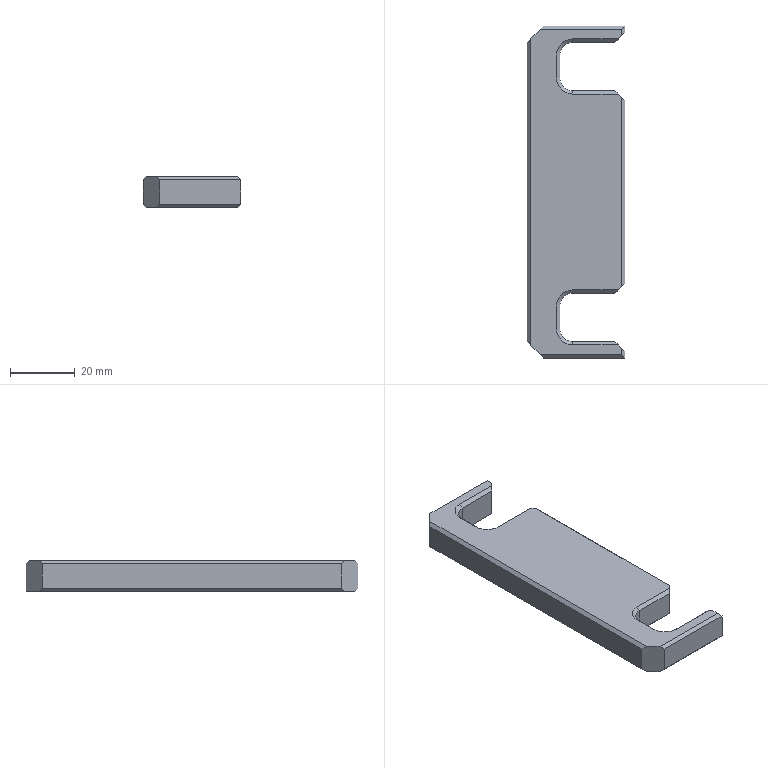Part | NX | features CHAMFER 3, DATUM_CSYS 3, EXTRUDE 3, BLEND 2, EXTRACT_STRING 2, SKETCH 2, Instance Feature 1, Pattern Feature 1 | 1 solid | 50 faces | box 30 x 102.4 x 9.5 mm | volume 22943 mm3 | plane 40 | cone 6 | cylinder 4 | commonest cylinder face diameters 8 x4
STEP:
#1=CARTESIAN_POINT('',(30.,23.,1.));
#2=VERTEX_POINT('',#1);
#3=CARTESIAN_POINT('',(30.,79.4,1.));
#4=VERTEX_POINT('',#3);
#5=CARTESIAN_POINT('',(30.,0.,1.));
#6=DIRECTION('',(0.,1.,0.));
#7=VECTOR('',#6,1000.);
#8=LINE('',#5,#7);
#9=EDGE_CURVE('',#2,#4,#8,.T.);
#10=ORIENTED_EDGE('',*,*,#9,.T.);
#11=CARTESIAN_POINT('',(30.,79.4,8.5));
#12=VERTEX_POINT('',#11);
#13=CARTESIAN_POINT('',(30.,79.4,8.5));
#14=DIRECTION('',(0.,0.,1.));
#15=VECTOR('',#14,1000.);
#16=LINE('',#13,#15);
#17=EDGE_CURVE('',#4,#12,#16,.T.);
#18=ORIENTED_EDGE('',*,*,#17,.T.);
#19=CARTESIAN_POINT('',(30.,23.,8.5));
#20=VERTEX_POINT('',#19);
#21=CARTESIAN_POINT('',(30.,0.,8.5));
#22=DIRECTION('',(0.,-1.,0.));
#23=VECTOR('',#22,1000.);
#24=LINE('',#21,#23);
#25=EDGE_CURVE('',#12,#20,#24,.T.);
#26=ORIENTED_EDGE('',*,*,#25,.T.);
#27=CARTESIAN_POINT('',(30.,23.,1.));
#28=DIRECTION('',(0.,0.,-1.));
#29=VECTOR('',#28,1000.);
#30=LINE('',#27,#29);
#31=EDGE_CURVE('',#20,#2,#30,.T.);
#32=ORIENTED_EDGE('',*,*,#31,.T.);
#33=EDGE_LOOP('',(#10,#18,#26,#32));
#34=FACE_BOUND('',#33,.T.);
#35=CARTESIAN_POINT('',(30.,0.,0.));
#36=DIRECTION('',(1.,0.,0.));
#37=DIRECTION('',(0.,0.,-1.));
#38=AXIS2_PLACEMENT_3D('',#35,#36,#37);
#39=PLANE('',#38);
#40=ADVANCED_FACE('',(#34),#39,.T.);
#41=CARTESIAN_POINT('',(30.,0.,1.));
#42=VERTEX_POINT('',#41);
#43=CARTESIAN_POINT('',(30.,2.,1.));
#44=VERTEX_POINT('',#43);
#45=CARTESIAN_POINT('',(30.,0.,1.));
#46=DIRECTION('',(0.,1.,0.));
#47=VECTOR('',#46,1000.);
#48=LINE('',#45,#47);
#49=EDGE_CURVE('',#42,#44,#48,.T.);
#50=ORIENTED_EDGE('',*,*,#49,.T.);
#51=CARTESIAN_POINT('',(30.,2.,8.5));
#52=VERTEX_POINT('',#51);
#53=CARTESIAN_POINT('',(30.,2.,8.5));
#54=DIRECTION('',(0.,0.,1.));
#55=VECTOR('',#54,1000.);
#56=LINE('',#53,#55);
#57=EDGE_CURVE('',#44,#52,#56,.T.);
#58=ORIENTED_EDGE('',*,*,#57,.T.);
#59=CARTESIAN_POINT('',(30.,0.,8.5));
#60=VERTEX_POINT('',#59);
#61=CARTESIAN_POINT('',(30.,0.,8.5));
#62=DIRECTION('',(0.,-1.,0.));
#63=VECTOR('',#62,1000.);
#64=LINE('',#61,#63);
#65=EDGE_CURVE('',#52,#60,#64,.T.);
#66=ORIENTED_EDGE('',*,*,#65,.T.);
#67=CARTESIAN_POINT('',(30.,0.,9.5));
#68=DIRECTION('',(0.,0.,-1.));
#69=VECTOR('',#68,1000.);
#70=LINE('',#67,#69);
#71=EDGE_CURVE('',#60,#42,#70,.T.);
#72=ORIENTED_EDGE('',*,*,#71,.T.);
#73=EDGE_LOOP('',(#50,#58,#66,#72));
#74=FACE_BOUND('',#73,.T.);
#75=CARTESIAN_POINT('',(30.,0.,0.));
#76=DIRECTION('',(1.,0.,0.));
#77=DIRECTION('',(0.,0.,-1.));
#78=AXIS2_PLACEMENT_3D('',#75,#76,#77);
#79=PLANE('',#78);
#80=ADVANCED_FACE('',(#74),#79,.T.);
#81=CARTESIAN_POINT('',(5.,0.,8.5));
#82=VERTEX_POINT('',#81);
#83=CARTESIAN_POINT('',(0.,0.,8.5));
#84=DIRECTION('',(-1.,0.,0.));
#85=VECTOR('',#84,1000.);
#86=LINE('',#83,#85);
#87=EDGE_CURVE('',#60,#82,#86,.T.);
#88=ORIENTED_EDGE('',*,*,#87,.T.);
#89=CARTESIAN_POINT('',(5.,0.,1.));
#90=VERTEX_POINT('',#89);
#91=CARTESIAN_POINT('',(5.,0.,1.));
#92=DIRECTION('',(0.,0.,-1.));
#93=VECTOR('',#92,1000.);
#94=LINE('',#91,#93);
#95=EDGE_CURVE('',#82,#90,#94,.T.);
#96=ORIENTED_EDGE('',*,*,#95,.T.);
#97=CARTESIAN_POINT('',(0.,0.,1.));
#98=DIRECTION('',(1.,0.,0.));
#99=VECTOR('',#98,1000.);
#100=LINE('',#97,#99);
#101=EDGE_CURVE('',#90,#42,#100,.T.);
#102=ORIENTED_EDGE('',*,*,#101,.T.);
#103=ORIENTED_EDGE('',*,*,#71,.F.);
#104=EDGE_LOOP('',(#88,#96,#102,#103));
#105=FACE_BOUND('',#104,.T.);
#106=CARTESIAN_POINT('',(0.,0.,9.5));
#107=DIRECTION('',(0.,-1.,0.));
#108=DIRECTION('',(0.,0.,-1.));
#109=AXIS2_PLACEMENT_3D('',#106,#107,#108);
#110=PLANE('',#109);
#111=ADVANCED_FACE('',(#105),#110,.T.);
#112=CARTESIAN_POINT('',(1.,4.,0.));
#113=VERTEX_POINT('',#112);
#114=CARTESIAN_POINT('',(1.,98.4,0.));
#115=VERTEX_POINT('',#114);
#116=CARTESIAN_POINT('',(1.,102.4,0.));
#117=DIRECTION('',(0.,1.,0.));
#118=VECTOR('',#117,1000.);
#119=LINE('',#116,#118);
#120=EDGE_CURVE('',#113,#115,#119,.T.);
#121=ORIENTED_EDGE('',*,*,#120,.T.);
#122=CARTESIAN_POINT('',(5.,102.4,0.));
#123=VERTEX_POINT('',#122);
#124=CARTESIAN_POINT('',(-48.7,48.7,0.));
#125=DIRECTION('',(0.7071,0.7071,0.));
#126=VECTOR('',#125,1000.);
#127=LINE('',#124,#126);
#128=EDGE_CURVE('',#115,#123,#127,.T.);
#129=ORIENTED_EDGE('',*,*,#128,.T.);
#130=CARTESIAN_POINT('',(29.,102.4,0.));
#131=VERTEX_POINT('',#130);
#132=CARTESIAN_POINT('',(0.,102.4,0.));
#133=DIRECTION('',(1.,0.,0.));
#134=VECTOR('',#133,1000.);
#135=LINE('',#132,#134);
#136=EDGE_CURVE('',#123,#131,#135,.T.);
#137=ORIENTED_EDGE('',*,*,#136,.T.);
#138=CARTESIAN_POINT('',(29.,99.4,0.));
#139=VERTEX_POINT('',#138);
#140=CARTESIAN_POINT('',(29.,0.,0.));
#141=DIRECTION('',(0.,-1.,0.));
#142=VECTOR('',#141,1000.);
#143=LINE('',#140,#142);
#144=EDGE_CURVE('',#131,#139,#143,.T.);
#145=ORIENTED_EDGE('',*,*,#144,.T.);
#146=CARTESIAN_POINT('',(27.,97.4,0.));
#147=VERTEX_POINT('',#146);
#148=CARTESIAN_POINT('',(-35.2,35.2,0.));
#149=DIRECTION('',(-0.7071,-0.7071,0.));
#150=VECTOR('',#149,1000.);
#151=LINE('',#148,#150);
#152=EDGE_CURVE('',#139,#147,#151,.T.);
#153=ORIENTED_EDGE('',*,*,#152,.T.);
#154=CARTESIAN_POINT('',(14.,97.4,0.));
#155=VERTEX_POINT('',#154);
#156=CARTESIAN_POINT('',(0.,97.4,0.));
#157=DIRECTION('',(1.,0.,0.));
#158=VECTOR('',#157,1000.);
#159=LINE('',#156,#158);
#160=EDGE_CURVE('',#155,#147,#159,.T.);
#161=ORIENTED_EDGE('',*,*,#160,.F.);
#162=CARTESIAN_POINT('',(10.,93.4,0.));
#163=VERTEX_POINT('',#162);
#164=CARTESIAN_POINT('',(14.,93.4,0.));
#165=DIRECTION('',(0.,0.,-1.));
#166=DIRECTION('',(0.,1.,0.));
#167=AXIS2_PLACEMENT_3D('',#164,#165,#166);
#168=CIRCLE('',#167,4.);
#169=EDGE_CURVE('',#155,#163,#168,.F.);
#170=ORIENTED_EDGE('',*,*,#169,.T.);
#171=CARTESIAN_POINT('',(10.,86.4,0.));
#172=VERTEX_POINT('',#171);
#173=CARTESIAN_POINT('',(10.,0.,0.));
#174=DIRECTION('',(0.,1.,0.));
#175=VECTOR('',#174,1000.);
#176=LINE('',#173,#175);
#177=EDGE_CURVE('',#172,#163,#176,.T.);
#178=ORIENTED_EDGE('',*,*,#177,.F.);
#179=CARTESIAN_POINT('',(14.,82.4,0.));
#180=VERTEX_POINT('',#179);
#181=CARTESIAN_POINT('',(14.,86.4,0.));
#182=DIRECTION('',(0.,0.,-1.));
#183=DIRECTION('',(0.,1.,0.));
#184=AXIS2_PLACEMENT_3D('',#181,#182,#183);
#185=CIRCLE('',#184,4.);
#186=EDGE_CURVE('',#172,#180,#185,.F.);
#187=ORIENTED_EDGE('',*,*,#186,.T.);
#188=CARTESIAN_POINT('',(27.,82.4,0.));
#189=VERTEX_POINT('',#188);
#190=CARTESIAN_POINT('',(0.,82.4,0.));
#191=DIRECTION('',(-1.,0.,0.));
#192=VECTOR('',#191,1000.);
#193=LINE('',#190,#192);
#194=EDGE_CURVE('',#189,#180,#193,.T.);
#195=ORIENTED_EDGE('',*,*,#194,.F.);
#196=CARTESIAN_POINT('',(29.,80.4,0.));
#197=VERTEX_POINT('',#196);
#198=CARTESIAN_POINT('',(54.7,54.7,0.));
#199=DIRECTION('',(0.7071,-0.7071,0.));
#200=VECTOR('',#199,1000.);
#201=LINE('',#198,#200);
#202=EDGE_CURVE('',#189,#197,#201,.T.);
#203=ORIENTED_EDGE('',*,*,#202,.T.);
#204=CARTESIAN_POINT('',(29.,22.,0.));
#205=VERTEX_POINT('',#204);
#206=CARTESIAN_POINT('',(29.,0.,0.));
#207=DIRECTION('',(0.,-1.,0.));
#208=VECTOR('',#207,1000.);
#209=LINE('',#206,#208);
#210=EDGE_CURVE('',#197,#205,#209,.T.);
#211=ORIENTED_EDGE('',*,*,#210,.T.);
#212=CARTESIAN_POINT('',(28.,21.,0.));
#213=VERTEX_POINT('',#212);
#214=CARTESIAN_POINT('',(3.5,-3.5,0.));
#215=DIRECTION('',(-0.7071,-0.7071,0.));
#216=VECTOR('',#215,1000.);
#217=LINE('',#214,#216);
#218=EDGE_CURVE('',#205,#213,#217,.T.);
#219=ORIENTED_EDGE('',*,*,#218,.T.);
#220=CARTESIAN_POINT('',(14.,21.,0.));
#221=VERTEX_POINT('',#220);
#222=CARTESIAN_POINT('',(14.,21.,0.));
#223=DIRECTION('',(-1.,0.,0.));
#224=VECTOR('',#223,1000.);
#225=LINE('',#222,#224);
#226=EDGE_CURVE('',#213,#221,#225,.T.);
#227=ORIENTED_EDGE('',*,*,#226,.T.);
#228=CARTESIAN_POINT('',(9.,16.,0.));
#229=VERTEX_POINT('',#228);
#230=CARTESIAN_POINT('',(14.,16.,0.));
#231=DIRECTION('',(0.,0.,-1.));
#232=DIRECTION('',(0.,1.,0.));
#233=AXIS2_PLACEMENT_3D('',#230,#231,#232);
#234=CIRCLE('',#233,5.);
#235=EDGE_CURVE('',#221,#229,#234,.F.);
#236=ORIENTED_EDGE('',*,*,#235,.T.);
#237=CARTESIAN_POINT('',(9.,9.,0.));
#238=VERTEX_POINT('',#237);
#239=CARTESIAN_POINT('',(9.,9.,0.));
#240=DIRECTION('',(0.,-1.,0.));
#241=VECTOR('',#240,1000.);
#242=LINE('',#239,#241);
#243=EDGE_CURVE('',#229,#238,#242,.T.);
#244=ORIENTED_EDGE('',*,*,#243,.T.);
#245=CARTESIAN_POINT('',(14.,4.,0.));
#246=VERTEX_POINT('',#245);
#247=CARTESIAN_POINT('',(14.,9.,0.));
#248=DIRECTION('',(0.,0.,-1.));
#249=DIRECTION('',(0.,1.,0.));
#250=AXIS2_PLACEMENT_3D('',#247,#248,#249);
#251=CIRCLE('',#250,5.);
#252=EDGE_CURVE('',#238,#246,#251,.F.);
#253=ORIENTED_EDGE('',*,*,#252,.T.);
#254=CARTESIAN_POINT('',(28.,4.,0.));
#255=VERTEX_POINT('',#254);
#256=CARTESIAN_POINT('',(30.,4.,0.));
#257=DIRECTION('',(1.,0.,0.));
#258=VECTOR('',#257,1000.);
#259=LINE('',#256,#258);
#260=EDGE_CURVE('',#246,#255,#259,.T.);
#261=ORIENTED_EDGE('',*,*,#260,.T.);
#262=CARTESIAN_POINT('',(29.,3.,0.));
#263=VERTEX_POINT('',#262);
#264=CARTESIAN_POINT('',(16.,16.,0.));
#265=DIRECTION('',(0.7071,-0.7071,0.));
#266=VECTOR('',#265,1000.);
#267=LINE('',#264,#266);
#268=EDGE_CURVE('',#255,#263,#267,.T.);
#269=ORIENTED_EDGE('',*,*,#268,.T.);
#270=CARTESIAN_POINT('',(29.,1.,0.));
#271=VERTEX_POINT('',#270);
#272=CARTESIAN_POINT('',(29.,0.,0.));
#273=DIRECTION('',(0.,-1.,0.));
#274=VECTOR('',#273,1000.);
#275=LINE('',#272,#274);
#276=EDGE_CURVE('',#263,#271,#275,.T.);
#277=ORIENTED_EDGE('',*,*,#276,.T.);
#278=CARTESIAN_POINT('',(4.,1.,0.));
#279=VERTEX_POINT('',#278);
#280=CARTESIAN_POINT('',(0.,1.,0.));
#281=DIRECTION('',(-1.,0.,0.));
#282=VECTOR('',#281,1000.);
#283=LINE('',#280,#282);
#284=EDGE_CURVE('',#271,#279,#283,.T.);
#285=ORIENTED_EDGE('',*,*,#284,.T.);
#286=CARTESIAN_POINT('',(2.5,2.5,0.));
#287=DIRECTION('',(-0.7071,0.7071,0.));
#288=VECTOR('',#287,1000.);
#289=LINE('',#286,#288);
#290=EDGE_CURVE('',#279,#113,#289,.T.);
#291=ORIENTED_EDGE('',*,*,#290,.T.);
#292=EDGE_LOOP('',(#121,#129,#137,#145,#153,#161,#170,#178,#187,#195,#203,#211,#219,#227,#236,#244,#253,#261,#269,#277,#285,#291));
#293=FACE_BOUND('',#292,.T.);
#294=CARTESIAN_POINT('',(0.,0.,0.));
#295=DIRECTION('',(0.,0.,-1.));
#296=DIRECTION('',(0.,1.,0.));
#297=AXIS2_PLACEMENT_3D('',#294,#295,#296);
#298=PLANE('',#297);
#299=ADVANCED_FACE('',(#293),#298,.T.);
#300=ORIENTED_EDGE('',*,*,#136,.F.);
#301=CARTESIAN_POINT('',(5.,102.4,8.5));
#302=VERTEX_POINT('',#301);
#303=CARTESIAN_POINT('',(5.,102.4,8.5));
#304=DIRECTION('',(0.,0.,1.));
#305=VECTOR('',#304,1000.);
#306=LINE('',#303,#305);
#307=EDGE_CURVE('',#123,#302,#306,.T.);
#308=ORIENTED_EDGE('',*,*,#307,.T.);
#309=CARTESIAN_POINT('',(30.,102.4,8.5));
#310=VERTEX_POINT('',#309);
#311=CARTESIAN_POINT('',(0.,102.4,8.5));
#312=DIRECTION('',(1.,0.,0.));
#313=VECTOR('',#312,1000.);
#314=LINE('',#311,#313);
#315=EDGE_CURVE('',#302,#310,#314,.T.);
#316=ORIENTED_EDGE('',*,*,#315,.T.);
#317=CARTESIAN_POINT('',(30.,102.4,1.));
#318=VERTEX_POINT('',#317);
#319=CARTESIAN_POINT('',(30.,102.4,0.));
#320=DIRECTION('',(0.,0.,1.));
#321=VECTOR('',#320,1000.);
#322=LINE('',#319,#321);
#323=EDGE_CURVE('',#318,#310,#322,.T.);
#324=ORIENTED_EDGE('',*,*,#323,.F.);
#325=CARTESIAN_POINT('',(14.5,102.4,-14.5));
#326=DIRECTION('',(0.7071,0.,0.7071));
#327=VECTOR('',#326,1000.);
#328=LINE('',#325,#327);
#329=EDGE_CURVE('',#318,#131,#328,.F.);
#330=ORIENTED_EDGE('',*,*,#329,.T.);
#331=EDGE_LOOP('',(#300,#308,#316,#324,#330));
#332=FACE_BOUND('',#331,.T.);
#333=CARTESIAN_POINT('',(0.,102.4,0.));
#334=DIRECTION('',(0.,1.,0.));
#335=DIRECTION('',(0.,0.,1.));
#336=AXIS2_PLACEMENT_3D('',#333,#334,#335);
#337=PLANE('',#336);
#338=ADVANCED_FACE('',(#332),#337,.T.);
#339=CARTESIAN_POINT('',(29.,101.4,9.5));
#340=VERTEX_POINT('',#339);
#341=CARTESIAN_POINT('',(4.,101.4,9.5));
#342=VERTEX_POINT('',#341);
#343=CARTESIAN_POINT('',(0.,101.4,9.5));
#344=DIRECTION('',(-1.,0.,0.));
#345=VECTOR('',#344,1000.);
#346=LINE('',#343,#345);
#347=EDGE_CURVE('',#340,#342,#346,.T.);
#348=ORIENTED_EDGE('',*,*,#347,.T.);
#349=CARTESIAN_POINT('',(1.,98.4,9.5));
#350=VERTEX_POINT('',#349);
#351=CARTESIAN_POINT('',(2.5,99.9,9.5));
#352=DIRECTION('',(-0.7071,-0.7071,0.));
#353=VECTOR('',#352,1000.);
#354=LINE('',#351,#353);
#355=EDGE_CURVE('',#342,#350,#354,.T.);
#356=ORIENTED_EDGE('',*,*,#355,.T.);
#357=CARTESIAN_POINT('',(1.,4.,9.5));
#358=VERTEX_POINT('',#357);
#359=CARTESIAN_POINT('',(1.,0.,9.5));
#360=DIRECTION('',(0.,-1.,0.));
#361=VECTOR('',#360,1000.);
#362=LINE('',#359,#361);
#363=EDGE_CURVE('',#350,#358,#362,.T.);
#364=ORIENTED_EDGE('',*,*,#363,.T.);
#365=CARTESIAN_POINT('',(4.,1.,9.5));
#366=VERTEX_POINT('',#365);
#367=CARTESIAN_POINT('',(-48.7,53.7,9.5));
#368=DIRECTION('',(0.7071,-0.7071,0.));
#369=VECTOR('',#368,1000.);
#370=LINE('',#367,#369);
#371=EDGE_CURVE('',#358,#366,#370,.T.);
#372=ORIENTED_EDGE('',*,*,#371,.T.);
#373=CARTESIAN_POINT('',(29.,1.,9.5));
#374=VERTEX_POINT('',#373);
#375=CARTESIAN_POINT('',(0.,1.,9.5));
#376=DIRECTION('',(1.,0.,0.));
#377=VECTOR('',#376,1000.);
#378=LINE('',#375,#377);
#379=EDGE_CURVE('',#366,#374,#378,.T.);
#380=ORIENTED_EDGE('',*,*,#379,.T.);
#381=CARTESIAN_POINT('',(29.,3.,9.5));
#382=VERTEX_POINT('',#381);
#383=CARTESIAN_POINT('',(29.,102.4,9.5));
#384=DIRECTION('',(0.,1.,0.));
#385=VECTOR('',#384,1000.);
#386=LINE('',#383,#385);
#387=EDGE_CURVE('',#374,#382,#386,.T.);
#388=ORIENTED_EDGE('',*,*,#387,.T.);
#389=CARTESIAN_POINT('',(28.,4.,9.5));
#390=VERTEX_POINT('',#389);
#391=CARTESIAN_POINT('',(-35.2,67.2,9.5));
#392=DIRECTION('',(-0.7071,0.7071,0.));
#393=VECTOR('',#392,1000.);
#394=LINE('',#391,#393);
#395=EDGE_CURVE('',#382,#390,#394,.T.);
#396=ORIENTED_EDGE('',*,*,#395,.T.);
#397=CARTESIAN_POINT('',(14.,4.,9.5));
#398=VERTEX_POINT('',#397);
#399=CARTESIAN_POINT('',(14.,4.,9.5));
#400=DIRECTION('',(-1.,0.,0.));
#401=VECTOR('',#400,1000.);
#402=LINE('',#399,#401);
#403=EDGE_CURVE('',#390,#398,#402,.T.);
#404=ORIENTED_EDGE('',*,*,#403,.T.);
#405=CARTESIAN_POINT('',(9.,9.,9.5));
#406=VERTEX_POINT('',#405);
#407=CARTESIAN_POINT('',(14.,9.,9.5));
#408=DIRECTION('',(0.,0.,1.));
#409=DIRECTION('',(0.,-1.,0.));
#410=AXIS2_PLACEMENT_3D('',#407,#408,#409);
#411=CIRCLE('',#410,5.);
#412=EDGE_CURVE('',#398,#406,#411,.F.);
#413=ORIENTED_EDGE('',*,*,#412,.T.);
#414=CARTESIAN_POINT('',(9.,16.,9.5));
#415=VERTEX_POINT('',#414);
#416=CARTESIAN_POINT('',(9.,16.,9.5));
#417=DIRECTION('',(0.,1.,0.));
#418=VECTOR('',#417,1000.);
#419=LINE('',#416,#418);
#420=EDGE_CURVE('',#406,#415,#419,.T.);
#421=ORIENTED_EDGE('',*,*,#420,.T.);
#422=CARTESIAN_POINT('',(14.,21.,9.5));
#423=VERTEX_POINT('',#422);
#424=CARTESIAN_POINT('',(14.,16.,9.5));
#425=DIRECTION('',(0.,0.,1.));
#426=DIRECTION('',(0.,-1.,0.));
#427=AXIS2_PLACEMENT_3D('',#424,#425,#426);
#428=CIRCLE('',#427,5.);
#429=EDGE_CURVE('',#415,#423,#428,.F.);
#430=ORIENTED_EDGE('',*,*,#429,.T.);
#431=CARTESIAN_POINT('',(28.,21.,9.5));
#432=VERTEX_POINT('',#431);
#433=CARTESIAN_POINT('',(30.,21.,9.5));
#434=DIRECTION('',(1.,0.,0.));
#435=VECTOR('',#434,1000.);
#436=LINE('',#433,#435);
#437=EDGE_CURVE('',#423,#432,#436,.T.);
#438=ORIENTED_EDGE('',*,*,#437,.T.);
#439=CARTESIAN_POINT('',(29.,22.,9.5));
#440=VERTEX_POINT('',#439);
#441=CARTESIAN_POINT('',(54.7,47.7,9.5));
#442=DIRECTION('',(0.7071,0.7071,0.));
#443=VECTOR('',#442,1000.);
#444=LINE('',#441,#443);
#445=EDGE_CURVE('',#432,#440,#444,.T.);
#446=ORIENTED_EDGE('',*,*,#445,.T.);
#447=CARTESIAN_POINT('',(29.,80.4,9.5));
#448=VERTEX_POINT('',#447);
#449=CARTESIAN_POINT('',(29.,102.4,9.5));
#450=DIRECTION('',(0.,1.,0.));
#451=VECTOR('',#450,1000.);
#452=LINE('',#449,#451);
#453=EDGE_CURVE('',#440,#448,#452,.T.);
#454=ORIENTED_EDGE('',*,*,#453,.T.);
#455=CARTESIAN_POINT('',(28.,81.4,9.5));
#456=VERTEX_POINT('',#455);
#457=CARTESIAN_POINT('',(3.5,105.9,9.5));
#458=DIRECTION('',(-0.7071,0.7071,0.));
#459=VECTOR('',#458,1000.);
#460=LINE('',#457,#459);
#461=EDGE_CURVE('',#448,#456,#460,.T.);
#462=ORIENTED_EDGE('',*,*,#461,.T.);
#463=CARTESIAN_POINT('',(14.,81.4,9.5));
#464=VERTEX_POINT('',#463);
#465=CARTESIAN_POINT('',(14.,81.4,9.5));
#466=DIRECTION('',(-1.,0.,0.));
#467=VECTOR('',#466,1000.);
#468=LINE('',#465,#467);
#469=EDGE_CURVE('',#456,#464,#468,.T.);
#470=ORIENTED_EDGE('',*,*,#469,.T.);
#471=CARTESIAN_POINT('',(9.,86.4,9.5));
#472=VERTEX_POINT('',#471);
#473=CARTESIAN_POINT('',(14.,86.4,9.5));
#474=DIRECTION('',(0.,0.,1.));
#475=DIRECTION('',(0.,-1.,0.));
#476=AXIS2_PLACEMENT_3D('',#473,#474,#475);
#477=CIRCLE('',#476,5.);
#478=EDGE_CURVE('',#464,#472,#477,.F.);
#479=ORIENTED_EDGE('',*,*,#478,.T.);
#480=CARTESIAN_POINT('',(9.,93.4,9.5));
#481=VERTEX_POINT('',#480);
#482=CARTESIAN_POINT('',(9.,93.4,9.5));
#483=DIRECTION('',(0.,1.,0.));
#484=VECTOR('',#483,1000.);
#485=LINE('',#482,#484);
#486=EDGE_CURVE('',#472,#481,#485,.T.);
#487=ORIENTED_EDGE('',*,*,#486,.T.);
#488=CARTESIAN_POINT('',(14.,98.4,9.5));
#489=VERTEX_POINT('',#488);
#490=CARTESIAN_POINT('',(14.,93.4,9.5));
#491=DIRECTION('',(0.,0.,1.));
#492=DIRECTION('',(0.,-1.,0.));
#493=AXIS2_PLACEMENT_3D('',#490,#491,#492);
#494=CIRCLE('',#493,5.);
#495=EDGE_CURVE('',#481,#489,#494,.F.);
#496=ORIENTED_EDGE('',*,*,#495,.T.);
#497=CARTESIAN_POINT('',(28.,98.4,9.5));
#498=VERTEX_POINT('',#497);
#499=CARTESIAN_POINT('',(30.,98.4,9.5));
#500=DIRECTION('',(1.,0.,0.));
#501=VECTOR('',#500,1000.);
#502=LINE('',#499,#501);
#503=EDGE_CURVE('',#489,#498,#502,.T.);
#504=ORIENTED_EDGE('',*,*,#503,.T.);
#505=CARTESIAN_POINT('',(29.,99.4,9.5));
#506=VERTEX_POINT('',#505);
#507=CARTESIAN_POINT('',(16.,86.4,9.5));
#508=DIRECTION('',(0.7071,0.7071,0.));
#509=VECTOR('',#508,1000.);
#510=LINE('',#507,#509);
#511=EDGE_CURVE('',#498,#506,#510,.T.);
#512=ORIENTED_EDGE('',*,*,#511,.T.);
#513=CARTESIAN_POINT('',(29.,102.4,9.5));
#514=DIRECTION('',(0.,1.,0.));
#515=VECTOR('',#514,1000.);
#516=LINE('',#513,#515);
#517=EDGE_CURVE('',#506,#340,#516,.T.);
#518=ORIENTED_EDGE('',*,*,#517,.T.);
#519=EDGE_LOOP('',(#348,#356,#364,#372,#380,#388,#396,#404,#413,#421,#430,#438,#446,#454,#462,#470,#479,#487,#496,#504,#512,#518));
#520=FACE_BOUND('',#519,.T.);
#521=CARTESIAN_POINT('',(0.,102.4,9.5));
#522=DIRECTION('',(0.,0.,1.));
#523=DIRECTION('',(0.,-1.,0.));
#524=AXIS2_PLACEMENT_3D('',#521,#522,#523);
#525=PLANE('',#524);
#526=ADVANCED_FACE('',(#520),#525,.T.);
#527=CARTESIAN_POINT('',(0.,5.,8.5));
#528=VERTEX_POINT('',#527);
#529=CARTESIAN_POINT('',(0.,97.4,8.5));
#530=VERTEX_POINT('',#529);
#531=CARTESIAN_POINT('',(0.,102.4,8.5));
#532=DIRECTION('',(0.,1.,0.));
#533=VECTOR('',#532,1000.);
#534=LINE('',#531,#533);
#535=EDGE_CURVE('',#528,#530,#534,.T.);
#536=ORIENTED_EDGE('',*,*,#535,.T.);
#537=CARTESIAN_POINT('',(0.,97.4,1.));
#538=VERTEX_POINT('',#537);
#539=CARTESIAN_POINT('',(0.,97.4,1.));
#540=DIRECTION('',(0.,0.,-1.));
#541=VECTOR('',#540,1000.);
#542=LINE('',#539,#541);
#543=EDGE_CURVE('',#530,#538,#542,.T.);
#544=ORIENTED_EDGE('',*,*,#543,.T.);
#545=CARTESIAN_POINT('',(0.,5.,1.));
#546=VERTEX_POINT('',#545);
#547=CARTESIAN_POINT('',(0.,0.,1.));
#548=DIRECTION('',(0.,-1.,0.));
#549=VECTOR('',#548,1000.);
#550=LINE('',#547,#549);
#551=EDGE_CURVE('',#538,#546,#550,.T.);
#552=ORIENTED_EDGE('',*,*,#551,.T.);
#553=CARTESIAN_POINT('',(0.,5.,8.5));
#554=DIRECTION('',(0.,0.,1.));
#555=VECTOR('',#554,1000.);
#556=LINE('',#553,#555);
#557=EDGE_CURVE('',#546,#528,#556,.T.);
#558=ORIENTED_EDGE('',*,*,#557,.T.);
#559=EDGE_LOOP('',(#536,#544,#552,#558));
#560=FACE_BOUND('',#559,.T.);
#561=CARTESIAN_POINT('',(0.,0.,0.));
#562=DIRECTION('',(1.,0.,0.));
#563=DIRECTION('',(0.,0.,-1.));
#564=AXIS2_PLACEMENT_3D('',#561,#562,#563);
#565=PLANE('',#564);
#566=ADVANCED_FACE('',(#560),#565,.F.);
#567=CARTESIAN_POINT('',(30.,100.4,8.5));
#568=VERTEX_POINT('',#567);
#569=CARTESIAN_POINT('',(30.,0.,8.5));
#570=DIRECTION('',(0.,-1.,0.));
#571=VECTOR('',#570,1000.);
#572=LINE('',#569,#571);
#573=EDGE_CURVE('',#310,#568,#572,.T.);
#574=ORIENTED_EDGE('',*,*,#573,.T.);
#575=CARTESIAN_POINT('',(30.,100.4,1.));
#576=VERTEX_POINT('',#575);
#577=CARTESIAN_POINT('',(30.,100.4,1.));
#578=DIRECTION('',(0.,0.,-1.));
#579=VECTOR('',#578,1000.);
#580=LINE('',#577,#579);
#581=EDGE_CURVE('',#568,#576,#580,.T.);
#582=ORIENTED_EDGE('',*,*,#581,.T.);
#583=CARTESIAN_POINT('',(30.,0.,1.));
#584=DIRECTION('',(0.,1.,0.));
#585=VECTOR('',#584,1000.);
#586=LINE('',#583,#585);
#587=EDGE_CURVE('',#576,#318,#586,.T.);
#588=ORIENTED_EDGE('',*,*,#587,.T.);
#589=ORIENTED_EDGE('',*,*,#323,.T.);
#590=EDGE_LOOP('',(#574,#582,#588,#589));
#591=FACE_BOUND('',#590,.T.);
#592=CARTESIAN_POINT('',(30.,0.,0.));
#593=DIRECTION('',(1.,0.,0.));
#594=DIRECTION('',(0.,0.,-1.));
#595=AXIS2_PLACEMENT_3D('',#592,#593,#594);
#596=PLANE('',#595);
#597=ADVANCED_FACE('',(#591),#596,.T.);
#598=CARTESIAN_POINT('',(10.,16.,1.));
#599=VERTEX_POINT('',#598);
#600=CARTESIAN_POINT('',(10.,16.,8.5));
#601=VERTEX_POINT('',#600);
#602=CARTESIAN_POINT('',(10.,16.,9.5));
#603=DIRECTION('',(0.,0.,-1.));
#604=VECTOR('',#603,1000.);
#605=LINE('',#602,#604);
#606=EDGE_CURVE('',#599,#601,#605,.F.);
#607=ORIENTED_EDGE('',*,*,#606,.T.);
#608=CARTESIAN_POINT('',(10.,9.,8.5));
#609=VERTEX_POINT('',#608);
#610=CARTESIAN_POINT('',(10.,9.,8.5));
#611=DIRECTION('',(0.,-1.,0.));
#612=VECTOR('',#611,1000.);
#613=LINE('',#610,#612);
#614=EDGE_CURVE('',#601,#609,#613,.T.);
#615=ORIENTED_EDGE('',*,*,#614,.T.);
#616=CARTESIAN_POINT('',(10.,9.,1.));
#617=VERTEX_POINT('',#616);
#618=CARTESIAN_POINT('',(10.,9.,0.));
#619=DIRECTION('',(0.,0.,-1.));
#620=VECTOR('',#619,1000.);
#621=LINE('',#618,#620);
#622=EDGE_CURVE('',#609,#617,#621,.T.);
#623=ORIENTED_EDGE('',*,*,#622,.T.);
#624=CARTESIAN_POINT('',(10.,16.,1.));
#625=DIRECTION('',(0.,1.,0.));
#626=VECTOR('',#625,1000.);
#627=LINE('',#624,#626);
#628=EDGE_CURVE('',#617,#599,#627,.T.);
#629=ORIENTED_EDGE('',*,*,#628,.T.);
#630=EDGE_LOOP('',(#607,#615,#623,#629));
#631=FACE_BOUND('',#630,.T.);
#632=CARTESIAN_POINT('',(10.,20.,-13.5));
#633=DIRECTION('',(-1.,0.,0.));
#634=DIRECTION('',(0.,-1.,0.));
#635=AXIS2_PLACEMENT_3D('',#632,#633,#634);
#636=PLANE('',#635);
#637=ADVANCED_FACE('',(#631),#636,.F.);
#638=CARTESIAN_POINT('',(14.,5.,8.5));
#639=VERTEX_POINT('',#638);
#640=CARTESIAN_POINT('',(27.,5.,8.5));
#641=VERTEX_POINT('',#640);
#642=CARTESIAN_POINT('',(30.,5.,8.5));
#643=DIRECTION('',(1.,0.,0.));
#644=VECTOR('',#643,1000.);
#645=LINE('',#642,#644);
#646=EDGE_CURVE('',#639,#641,#645,.T.);
#647=ORIENTED_EDGE('',*,*,#646,.T.);
#648=CARTESIAN_POINT('',(27.,5.,1.));
#649=VERTEX_POINT('',#648);
#650=CARTESIAN_POINT('',(27.,5.,1.));
#651=DIRECTION('',(0.,0.,-1.));
#652=VECTOR('',#651,1000.);
#653=LINE('',#650,#652);
#654=EDGE_CURVE('',#641,#649,#653,.T.);
#655=ORIENTED_EDGE('',*,*,#654,.T.);
#656=CARTESIAN_POINT('',(14.,5.,1.));
#657=VERTEX_POINT('',#656);
#658=CARTESIAN_POINT('',(14.,5.,1.));
#659=DIRECTION('',(-1.,0.,0.));
#660=VECTOR('',#659,1000.);
#661=LINE('',#658,#660);
#662=EDGE_CURVE('',#649,#657,#661,.T.);
#663=ORIENTED_EDGE('',*,*,#662,.T.);
#664=CARTESIAN_POINT('',(14.,5.,9.5));
#665=DIRECTION('',(0.,0.,-1.));
#666=VECTOR('',#665,1000.);
#667=LINE('',#664,#666);
#668=EDGE_CURVE('',#657,#639,#667,.F.);
#669=ORIENTED_EDGE('',*,*,#668,.T.);
#670=EDGE_LOOP('',(#647,#655,#663,#669));
#671=FACE_BOUND('',#670,.T.);
#672=CARTESIAN_POINT('',(10.,5.,-13.5));
#673=DIRECTION('',(0.,-1.,0.));
#674=DIRECTION('',(1.,0.,0.));
#675=AXIS2_PLACEMENT_3D('',#672,#673,#674);
#676=PLANE('',#675);
#677=ADVANCED_FACE('',(#671),#676,.F.);
#678=CARTESIAN_POINT('',(14.,20.,1.));
#679=VERTEX_POINT('',#678);
#680=CARTESIAN_POINT('',(27.,20.,1.));
#681=VERTEX_POINT('',#680);
#682=CARTESIAN_POINT('',(30.,20.,1.));
#683=DIRECTION('',(1.,0.,0.));
#684=VECTOR('',#683,1000.);
#685=LINE('',#682,#684);
#686=EDGE_CURVE('',#679,#681,#685,.T.);
#687=ORIENTED_EDGE('',*,*,#686,.T.);
#688=CARTESIAN_POINT('',(27.,20.,8.5));
#689=VERTEX_POINT('',#688);
#690=CARTESIAN_POINT('',(27.,20.,8.5));
#691=DIRECTION('',(0.,0.,1.));
#692=VECTOR('',#691,1000.);
#693=LINE('',#690,#692);
#694=EDGE_CURVE('',#681,#689,#693,.T.);
#695=ORIENTED_EDGE('',*,*,#694,.T.);
#696=CARTESIAN_POINT('',(14.,20.,8.5));
#697=VERTEX_POINT('',#696);
#698=CARTESIAN_POINT('',(14.,20.,8.5));
#699=DIRECTION('',(-1.,0.,0.));
#700=VECTOR('',#699,1000.);
#701=LINE('',#698,#700);
#702=EDGE_CURVE('',#689,#697,#701,.T.);
#703=ORIENTED_EDGE('',*,*,#702,.T.);
#704=CARTESIAN_POINT('',(14.,20.,0.));
#705=DIRECTION('',(0.,0.,-1.));
#706=VECTOR('',#705,1000.);
#707=LINE('',#704,#706);
#708=EDGE_CURVE('',#697,#679,#707,.T.);
#709=ORIENTED_EDGE('',*,*,#708,.T.);
#710=EDGE_LOOP('',(#687,#695,#703,#709));
#711=FACE_BOUND('',#710,.T.);
#712=CARTESIAN_POINT('',(35.5,20.,-13.5));
#713=DIRECTION('',(0.,1.,0.));
#714=DIRECTION('',(-1.,0.,0.));
#715=AXIS2_PLACEMENT_3D('',#712,#713,#714);
#716=PLANE('',#715);
#717=ADVANCED_FACE('',(#711),#716,.F.);
#718=ORIENTED_EDGE('',*,*,#708,.F.);
#719=CARTESIAN_POINT('',(14.,16.,8.5));
#720=DIRECTION('',(0.,0.,1.));
#721=DIRECTION('',(1.,0.,0.));
#722=AXIS2_PLACEMENT_3D('',#719,#720,#721);
#723=CIRCLE('',#722,4.);
#724=EDGE_CURVE('',#697,#601,#723,.T.);
#725=ORIENTED_EDGE('',*,*,#724,.T.);
#726=ORIENTED_EDGE('',*,*,#606,.F.);
#727=CARTESIAN_POINT('',(14.,16.,1.));
#728=DIRECTION('',(0.,0.,-1.));
#729=DIRECTION('',(-1.,0.,0.));
#730=AXIS2_PLACEMENT_3D('',#727,#728,#729);
#731=CIRCLE('',#730,4.);
#732=EDGE_CURVE('',#599,#679,#731,.T.);
#733=ORIENTED_EDGE('',*,*,#732,.T.);
#734=EDGE_LOOP('',(#718,#725,#726,#733));
#735=FACE_BOUND('',#734,.T.);
#736=CARTESIAN_POINT('',(14.,16.,-13.5));
#737=DIRECTION('',(0.,0.,1.));
#738=DIRECTION('',(0.,-1.,0.));
#739=AXIS2_PLACEMENT_3D('',#736,#737,#738);
#740=CYLINDRICAL_SURFACE('',#739,4.);
#741=ADVANCED_FACE('',(#735),#740,.F.);
#742=ORIENTED_EDGE('',*,*,#622,.F.);
#743=CARTESIAN_POINT('',(14.,9.,8.5));
#744=DIRECTION('',(0.,0.,1.));
#745=DIRECTION('',(1.,0.,0.));
#746=AXIS2_PLACEMENT_3D('',#743,#744,#745);
#747=CIRCLE('',#746,4.);
#748=EDGE_CURVE('',#609,#639,#747,.T.);
#749=ORIENTED_EDGE('',*,*,#748,.T.);
#750=ORIENTED_EDGE('',*,*,#668,.F.);
#751=CARTESIAN_POINT('',(14.,9.,1.));
#752=DIRECTION('',(0.,0.,-1.));
#753=DIRECTION('',(-1.,0.,0.));
#754=AXIS2_PLACEMENT_3D('',#751,#752,#753);
#755=CIRCLE('',#754,4.);
#756=EDGE_CURVE('',#657,#617,#755,.T.);
#757=ORIENTED_EDGE('',*,*,#756,.T.);
#758=EDGE_LOOP('',(#742,#749,#750,#757));
#759=FACE_BOUND('',#758,.T.);
#760=CARTESIAN_POINT('',(14.,9.,-13.5));
#761=DIRECTION('',(0.,0.,1.));
#762=DIRECTION('',(0.,-1.,0.));
#763=AXIS2_PLACEMENT_3D('',#760,#761,#762);
#764=CYLINDRICAL_SURFACE('',#763,4.);
#765=ADVANCED_FACE('',(#759),#764,.F.);
#766=CARTESIAN_POINT('',(10.,93.4,8.5));
#767=VERTEX_POINT('',#766);
#768=CARTESIAN_POINT('',(10.,93.4,9.5));
#769=DIRECTION('',(0.,0.,-1.));
#770=VECTOR('',#769,1000.);
#771=LINE('',#768,#770);
#772=EDGE_CURVE('',#163,#767,#771,.F.);
#773=ORIENTED_EDGE('',*,*,#772,.T.);
#774=CARTESIAN_POINT('',(10.,86.4,8.5));
#775=VERTEX_POINT('',#774);
#776=CARTESIAN_POINT('',(10.,86.4,8.5));
#777=DIRECTION('',(0.,-1.,0.));
#778=VECTOR('',#777,1000.);
#779=LINE('',#776,#778);
#780=EDGE_CURVE('',#767,#775,#779,.T.);
#781=ORIENTED_EDGE('',*,*,#780,.T.);
#782=CARTESIAN_POINT('',(10.,86.4,0.));
#783=DIRECTION('',(0.,0.,-1.));
#784=VECTOR('',#783,1000.);
#785=LINE('',#782,#784);
#786=EDGE_CURVE('',#775,#172,#785,.T.);
#787=ORIENTED_EDGE('',*,*,#786,.T.);
#788=ORIENTED_EDGE('',*,*,#177,.T.);
#789=EDGE_LOOP('',(#773,#781,#787,#788));
#790=FACE_BOUND('',#789,.T.);
#791=CARTESIAN_POINT('',(10.,97.4,-13.5));
#792=DIRECTION('',(-1.,0.,0.));
#793=DIRECTION('',(0.,-1.,0.));
#794=AXIS2_PLACEMENT_3D('',#791,#792,#793);
#795=PLANE('',#794);
#796=ADVANCED_FACE('',(#790),#795,.F.);
#797=CARTESIAN_POINT('',(14.,82.4,8.5));
#798=VERTEX_POINT('',#797);
#799=CARTESIAN_POINT('',(27.,82.4,8.5));
#800=VERTEX_POINT('',#799);
#801=CARTESIAN_POINT('',(30.,82.4,8.5));
#802=DIRECTION('',(1.,0.,0.));
#803=VECTOR('',#802,1000.);
#804=LINE('',#801,#803);
#805=EDGE_CURVE('',#798,#800,#804,.T.);
#806=ORIENTED_EDGE('',*,*,#805,.T.);
#807=CARTESIAN_POINT('',(27.,82.4,1.));
#808=DIRECTION('',(0.,0.,-1.));
#809=VECTOR('',#808,1000.);
#810=LINE('',#807,#809);
#811=EDGE_CURVE('',#800,#189,#810,.T.);
#812=ORIENTED_EDGE('',*,*,#811,.T.);
#813=ORIENTED_EDGE('',*,*,#194,.T.);
#814=CARTESIAN_POINT('',(14.,82.4,9.5));
#815=DIRECTION('',(0.,0.,-1.));
#816=VECTOR('',#815,1000.);
#817=LINE('',#814,#816);
#818=EDGE_CURVE('',#180,#798,#817,.F.);
#819=ORIENTED_EDGE('',*,*,#818,.T.);
#820=EDGE_LOOP('',(#806,#812,#813,#819));
#821=FACE_BOUND('',#820,.T.);
#822=CARTESIAN_POINT('',(10.,82.4,-13.5));
#823=DIRECTION('',(0.,-1.,0.));
#824=DIRECTION('',(0.,0.,-1.));
#825=AXIS2_PLACEMENT_3D('',#822,#823,#824);
#826=PLANE('',#825);
#827=ADVANCED_FACE('',(#821),#826,.F.);
#828=ORIENTED_EDGE('',*,*,#160,.T.);
#829=CARTESIAN_POINT('',(27.,97.4,8.5));
#830=VERTEX_POINT('',#829);
#831=CARTESIAN_POINT('',(27.,97.4,8.5));
#832=DIRECTION('',(0.,0.,1.));
#833=VECTOR('',#832,1000.);
#834=LINE('',#831,#833);
#835=EDGE_CURVE('',#147,#830,#834,.T.);
#836=ORIENTED_EDGE('',*,*,#835,.T.);
#837=CARTESIAN_POINT('',(14.,97.4,8.5));
#838=VERTEX_POINT('',#837);
#839=CARTESIAN_POINT('',(14.,97.4,8.5));
#840=DIRECTION('',(-1.,0.,0.));
#841=VECTOR('',#840,1000.);
#842=LINE('',#839,#841);
#843=EDGE_CURVE('',#830,#838,#842,.T.);
#844=ORIENTED_EDGE('',*,*,#843,.T.);
#845=CARTESIAN_POINT('',(14.,97.4,0.));
#846=DIRECTION('',(0.,0.,-1.));
#847=VECTOR('',#846,1000.);
#848=LINE('',#845,#847);
#849=EDGE_CURVE('',#838,#155,#848,.T.);
#850=ORIENTED_EDGE('',*,*,#849,.T.);
#851=EDGE_LOOP('',(#828,#836,#844,#850));
#852=FACE_BOUND('',#851,.T.);
#853=CARTESIAN_POINT('',(35.5,97.4,-13.5));
#854=DIRECTION('',(0.,1.,0.));
#855=DIRECTION('',(-1.,0.,0.));
#856=AXIS2_PLACEMENT_3D('',#853,#854,#855);
#857=PLANE('',#856);
#858=ADVANCED_FACE('',(#852),#857,.F.);
#859=ORIENTED_EDGE('',*,*,#849,.F.);
#860=CARTESIAN_POINT('',(14.,93.4,8.5));
#861=DIRECTION('',(0.,0.,1.));
#862=DIRECTION('',(1.,0.,0.));
#863=AXIS2_PLACEMENT_3D('',#860,#861,#862);
#864=CIRCLE('',#863,4.);
#865=EDGE_CURVE('',#838,#767,#864,.T.);
#866=ORIENTED_EDGE('',*,*,#865,.T.);
#867=ORIENTED_EDGE('',*,*,#772,.F.);
#868=ORIENTED_EDGE('',*,*,#169,.F.);
#869=EDGE_LOOP('',(#859,#866,#867,#868));
#870=FACE_BOUND('',#869,.T.);
#871=CARTESIAN_POINT('',(14.,93.4,-13.5));
#872=DIRECTION('',(0.,0.,1.));
#873=DIRECTION('',(0.,-1.,0.));
#874=AXIS2_PLACEMENT_3D('',#871,#872,#873);
#875=CYLINDRICAL_SURFACE('',#874,4.);
#876=ADVANCED_FACE('',(#870),#875,.F.);
#877=ORIENTED_EDGE('',*,*,#786,.F.);
#878=CARTESIAN_POINT('',(14.,86.4,8.5));
#879=DIRECTION('',(0.,0.,1.));
#880=DIRECTION('',(1.,0.,0.));
#881=AXIS2_PLACEMENT_3D('',#878,#879,#880);
#882=CIRCLE('',#881,4.);
#883=EDGE_CURVE('',#775,#798,#882,.T.);
#884=ORIENTED_EDGE('',*,*,#883,.T.);
#885=ORIENTED_EDGE('',*,*,#818,.F.);
#886=ORIENTED_EDGE('',*,*,#186,.F.);
#887=EDGE_LOOP('',(#877,#884,#885,#886));
#888=FACE_BOUND('',#887,.T.);
#889=CARTESIAN_POINT('',(14.,86.4,-13.5));
#890=DIRECTION('',(0.,0.,1.));
#891=DIRECTION('',(0.,-1.,0.));
#892=AXIS2_PLACEMENT_3D('',#889,#890,#891);
#893=CYLINDRICAL_SURFACE('',#892,4.);
#894=ADVANCED_FACE('',(#888),#893,.F.);
#895=CARTESIAN_POINT('',(9.,93.4,9.5));
#896=DIRECTION('',(0.7071,0.,-0.7071));
#897=VECTOR('',#896,1000.);
#898=LINE('',#895,#897);
#899=EDGE_CURVE('',#481,#767,#898,.T.);
#900=ORIENTED_EDGE('',*,*,#899,.F.);
#901=ORIENTED_EDGE('',*,*,#486,.F.);
#902=CARTESIAN_POINT('',(10.,86.4,8.5));
#903=DIRECTION('',(-0.7071,0.,0.7071));
#904=VECTOR('',#903,1000.);
#905=LINE('',#902,#904);
#906=EDGE_CURVE('',#775,#472,#905,.T.);
#907=ORIENTED_EDGE('',*,*,#906,.F.);
#908=ORIENTED_EDGE('',*,*,#780,.F.);
#909=EDGE_LOOP('',(#900,#901,#907,#908));
#910=FACE_BOUND('',#909,.T.);
#911=CARTESIAN_POINT('',(10.,97.4,8.5));
#912=DIRECTION('',(0.7071,0.,0.7071));
#913=DIRECTION('',(0.,1.,0.));
#914=AXIS2_PLACEMENT_3D('',#911,#912,#913);
#915=PLANE('',#914);
#916=ADVANCED_FACE('',(#910),#915,.T.);
#917=ORIENTED_EDGE('',*,*,#906,.T.);
#918=ORIENTED_EDGE('',*,*,#478,.F.);
#919=CARTESIAN_POINT('',(14.,82.4,8.5));
#920=DIRECTION('',(0.,-0.7071,0.7071));
#921=VECTOR('',#920,1000.);
#922=LINE('',#919,#921);
#923=EDGE_CURVE('',#798,#464,#922,.T.);
#924=ORIENTED_EDGE('',*,*,#923,.F.);
#925=ORIENTED_EDGE('',*,*,#883,.F.);
#926=EDGE_LOOP('',(#917,#918,#924,#925));
#927=FACE_BOUND('',#926,.T.);
#928=CARTESIAN_POINT('',(14.,86.4,9.5));
#929=DIRECTION('',(0.,0.,1.));
#930=DIRECTION('',(1.,0.,0.));
#931=AXIS2_PLACEMENT_3D('',#928,#929,#930);
#932=CONICAL_SURFACE('',#931,5.,0.7854);
#933=ADVANCED_FACE('',(#927),#932,.F.);
#934=ORIENTED_EDGE('',*,*,#899,.T.);
#935=ORIENTED_EDGE('',*,*,#865,.F.);
#936=CARTESIAN_POINT('',(14.,98.4,9.5));
#937=DIRECTION('',(0.,-0.7071,-0.7071));
#938=VECTOR('',#937,1000.);
#939=LINE('',#936,#938);
#940=EDGE_CURVE('',#489,#838,#939,.T.);
#941=ORIENTED_EDGE('',*,*,#940,.F.);
#942=ORIENTED_EDGE('',*,*,#495,.F.);
#943=EDGE_LOOP('',(#934,#935,#941,#942));
#944=FACE_BOUND('',#943,.T.);
#945=CARTESIAN_POINT('',(14.,93.4,9.5));
#946=DIRECTION('',(0.,0.,1.));
#947=DIRECTION('',(1.,0.,0.));
#948=AXIS2_PLACEMENT_3D('',#945,#946,#947);
#949=CONICAL_SURFACE('',#948,5.,0.7854);
#950=ADVANCED_FACE('',(#944),#949,.F.);
#951=ORIENTED_EDGE('',*,*,#469,.F.);
#952=CARTESIAN_POINT('',(21.333,88.067,2.833));
#953=DIRECTION('',(-0.5774,0.5774,-0.5774));
#954=VECTOR('',#953,1000.);
#955=LINE('',#952,#954);
#956=EDGE_CURVE('',#456,#800,#955,.T.);
#957=ORIENTED_EDGE('',*,*,#956,.T.);
#958=ORIENTED_EDGE('',*,*,#805,.F.);
#959=ORIENTED_EDGE('',*,*,#923,.T.);
#960=EDGE_LOOP('',(#951,#957,#958,#959));
#961=FACE_BOUND('',#960,.T.);
#962=CARTESIAN_POINT('',(10.,82.4,8.5));
#963=DIRECTION('',(0.,0.7071,0.7071));
#964=DIRECTION('',(-1.,0.,0.));
#965=AXIS2_PLACEMENT_3D('',#962,#963,#964);
#966=PLANE('',#965);
#967=ADVANCED_FACE('',(#961),#966,.T.);
#968=ORIENTED_EDGE('',*,*,#843,.F.);
#969=CARTESIAN_POINT('',(29.833,100.233,11.333));
#970=DIRECTION('',(0.5774,0.5774,0.5774));
#971=VECTOR('',#970,1000.);
#972=LINE('',#969,#971);
#973=EDGE_CURVE('',#830,#498,#972,.T.);
#974=ORIENTED_EDGE('',*,*,#973,.T.);
#975=ORIENTED_EDGE('',*,*,#503,.F.);
#976=ORIENTED_EDGE('',*,*,#940,.T.);
#977=EDGE_LOOP('',(#968,#974,#975,#976));
#978=FACE_BOUND('',#977,.T.);
#979=CARTESIAN_POINT('',(35.5,97.4,8.5));
#980=DIRECTION('',(0.,-0.7071,0.7071));
#981=DIRECTION('',(1.,0.,0.));
#982=AXIS2_PLACEMENT_3D('',#979,#980,#981);
#983=PLANE('',#982);
#984=ADVANCED_FACE('',(#978),#983,.T.);
#985=ORIENTED_EDGE('',*,*,#25,.F.);
#986=CARTESIAN_POINT('',(56.467,52.933,-17.967));
#987=DIRECTION('',(0.5774,-0.5774,-0.5774));
#988=VECTOR('',#987,1000.);
#989=LINE('',#986,#988);
#990=EDGE_CURVE('',#12,#448,#989,.F.);
#991=ORIENTED_EDGE('',*,*,#990,.T.);
#992=ORIENTED_EDGE('',*,*,#453,.F.);
#993=CARTESIAN_POINT('',(22.333,15.333,16.167));
#994=DIRECTION('',(-0.5774,-0.5774,0.5774));
#995=VECTOR('',#994,1000.);
#996=LINE('',#993,#995);
#997=EDGE_CURVE('',#440,#20,#996,.F.);
#998=ORIENTED_EDGE('',*,*,#997,.T.);
#999=EDGE_LOOP('',(#985,#991,#992,#998));
#1000=FACE_BOUND('',#999,.T.);
#1001=CARTESIAN_POINT('',(30.,0.,8.5));
#1002=DIRECTION('',(-0.7071,0.,-0.7071));
#1003=DIRECTION('',(0.,-1.,0.));
#1004=AXIS2_PLACEMENT_3D('',#1001,#1002,#1003);
#1005=PLANE('',#1004);
#1006=ADVANCED_FACE('',(#1000),#1005,.F.);
#1007=ORIENTED_EDGE('',*,*,#517,.F.);
#1008=CARTESIAN_POINT('',(-3.467,66.933,41.967));
#1009=DIRECTION('',(-0.5774,-0.5774,0.5774));
#1010=VECTOR('',#1009,1000.);
#1011=LINE('',#1008,#1010);
#1012=EDGE_CURVE('',#506,#568,#1011,.F.);
#1013=ORIENTED_EDGE('',*,*,#1012,.T.);
#1014=ORIENTED_EDGE('',*,*,#573,.F.);
#1015=CARTESIAN_POINT('',(-4.133,68.267,42.633));
#1016=DIRECTION('',(-0.5774,-0.5774,0.5774));
#1017=VECTOR('',#1016,1000.);
#1018=LINE('',#1015,#1017);
#1019=EDGE_CURVE('',#340,#310,#1018,.F.);
#1020=ORIENTED_EDGE('',*,*,#1019,.F.);
#1021=EDGE_LOOP('',(#1007,#1013,#1014,#1020));
#1022=FACE_BOUND('',#1021,.T.);
#1023=CARTESIAN_POINT('',(30.,0.,8.5));
#1024=DIRECTION('',(-0.7071,0.,-0.7071));
#1025=DIRECTION('',(0.,-1.,0.));
#1026=AXIS2_PLACEMENT_3D('',#1023,#1024,#1025);
#1027=PLANE('',#1026);
#1028=ADVANCED_FACE('',(#1022),#1027,.F.);
#1029=ORIENTED_EDGE('',*,*,#702,.F.);
#1030=CARTESIAN_POINT('',(29.833,22.833,11.333));
#1031=DIRECTION('',(0.5774,0.5774,0.5774));
#1032=VECTOR('',#1031,1000.);
#1033=LINE('',#1030,#1032);
#1034=EDGE_CURVE('',#689,#432,#1033,.T.);
#1035=ORIENTED_EDGE('',*,*,#1034,.T.);
#1036=ORIENTED_EDGE('',*,*,#437,.F.);
#1037=CARTESIAN_POINT('',(14.,20.,8.5));
#1038=DIRECTION('',(0.,0.7071,0.7071));
#1039=VECTOR('',#1038,1000.);
#1040=LINE('',#1037,#1039);
#1041=EDGE_CURVE('',#697,#423,#1040,.T.);
#1042=ORIENTED_EDGE('',*,*,#1041,.F.);
#1043=EDGE_LOOP('',(#1029,#1035,#1036,#1042));
#1044=FACE_BOUND('',#1043,.T.);
#1045=CARTESIAN_POINT('',(35.5,20.,8.5));
#1046=DIRECTION('',(0.,-0.7071,0.7071));
#1047=DIRECTION('',(1.,0.,0.));
#1048=AXIS2_PLACEMENT_3D('',#1045,#1046,#1047);
#1049=PLANE('',#1048);
#1050=ADVANCED_FACE('',(#1044),#1049,.T.);
#1051=ORIENTED_EDGE('',*,*,#315,.F.);
#1052=CARTESIAN_POINT('',(3.333,100.733,10.167));
#1053=DIRECTION('',(0.5774,0.5774,-0.5774));
#1054=VECTOR('',#1053,1000.);
#1055=LINE('',#1052,#1054);
#1056=EDGE_CURVE('',#302,#342,#1055,.F.);
#1057=ORIENTED_EDGE('',*,*,#1056,.T.);
#1058=ORIENTED_EDGE('',*,*,#347,.F.);
#1059=ORIENTED_EDGE('',*,*,#1019,.T.);
#1060=EDGE_LOOP('',(#1051,#1057,#1058,#1059));
#1061=FACE_BOUND('',#1060,.T.);
#1062=CARTESIAN_POINT('',(0.,102.4,8.5));
#1063=DIRECTION('',(0.,-0.7071,-0.7071));
#1064=DIRECTION('',(1.,0.,0.));
#1065=AXIS2_PLACEMENT_3D('',#1062,#1063,#1064);
#1066=PLANE('',#1065);
#1067=ADVANCED_FACE('',(#1061),#1066,.F.);
#1068=ORIENTED_EDGE('',*,*,#1041,.T.);
#1069=ORIENTED_EDGE('',*,*,#429,.F.);
#1070=CARTESIAN_POINT('',(10.,16.,8.5));
#1071=DIRECTION('',(-0.7071,0.,0.7071));
#1072=VECTOR('',#1071,1000.);
#1073=LINE('',#1070,#1072);
#1074=EDGE_CURVE('',#601,#415,#1073,.T.);
#1075=ORIENTED_EDGE('',*,*,#1074,.F.);
#1076=ORIENTED_EDGE('',*,*,#724,.F.);
#1077=EDGE_LOOP('',(#1068,#1069,#1075,#1076));
#1078=FACE_BOUND('',#1077,.T.);
#1079=CARTESIAN_POINT('',(14.,16.,9.5));
#1080=DIRECTION('',(0.,0.,1.));
#1081=DIRECTION('',(1.,0.,0.));
#1082=AXIS2_PLACEMENT_3D('',#1079,#1080,#1081);
#1083=CONICAL_SURFACE('',#1082,5.,0.7854);
#1084=ADVANCED_FACE('',(#1078),#1083,.F.);
#1085=ORIENTED_EDGE('',*,*,#363,.F.);
#1086=CARTESIAN_POINT('',(2.333,99.733,10.833));
#1087=DIRECTION('',(-0.5774,-0.5774,-0.5774));
#1088=VECTOR('',#1087,1000.);
#1089=LINE('',#1086,#1088);
#1090=EDGE_CURVE('',#350,#530,#1089,.T.);
#1091=ORIENTED_EDGE('',*,*,#1090,.T.);
#1092=ORIENTED_EDGE('',*,*,#535,.F.);
#1093=CARTESIAN_POINT('',(-31.8,36.8,-23.3));
#1094=DIRECTION('',(0.5774,-0.5774,0.5774));
#1095=VECTOR('',#1094,1000.);
#1096=LINE('',#1093,#1095);
#1097=EDGE_CURVE('',#528,#358,#1096,.T.);
#1098=ORIENTED_EDGE('',*,*,#1097,.T.);
#1099=EDGE_LOOP('',(#1085,#1091,#1092,#1098));
#1100=FACE_BOUND('',#1099,.T.);
#1101=CARTESIAN_POINT('',(1.,102.4,9.5));
#1102=DIRECTION('',(-0.7071,0.,0.7071));
#1103=DIRECTION('',(0.,1.,0.));
#1104=AXIS2_PLACEMENT_3D('',#1101,#1102,#1103);
#1105=PLANE('',#1104);
#1106=ADVANCED_FACE('',(#1100),#1105,.T.);
#1107=ORIENTED_EDGE('',*,*,#1074,.T.);
#1108=ORIENTED_EDGE('',*,*,#420,.F.);
#1109=CARTESIAN_POINT('',(10.,9.,8.5));
#1110=DIRECTION('',(-0.7071,0.,0.7071));
#1111=VECTOR('',#1110,1000.);
#1112=LINE('',#1109,#1111);
#1113=EDGE_CURVE('',#609,#406,#1112,.T.);
#1114=ORIENTED_EDGE('',*,*,#1113,.F.);
#1115=ORIENTED_EDGE('',*,*,#614,.F.);
#1116=EDGE_LOOP('',(#1107,#1108,#1114,#1115));
#1117=FACE_BOUND('',#1116,.T.);
#1118=CARTESIAN_POINT('',(10.,20.,8.5));
#1119=DIRECTION('',(0.7071,0.,0.7071));
#1120=DIRECTION('',(0.,1.,0.));
#1121=AXIS2_PLACEMENT_3D('',#1118,#1119,#1120);
#1122=PLANE('',#1121);
#1123=ADVANCED_FACE('',(#1117),#1122,.T.);
#1124=ORIENTED_EDGE('',*,*,#379,.F.);
#1125=CARTESIAN_POINT('',(2.667,2.333,10.833));
#1126=DIRECTION('',(-0.5774,0.5774,0.5774));
#1127=VECTOR('',#1126,1000.);
#1128=LINE('',#1125,#1127);
#1129=EDGE_CURVE('',#366,#82,#1128,.F.);
#1130=ORIENTED_EDGE('',*,*,#1129,.T.);
#1131=ORIENTED_EDGE('',*,*,#87,.F.);
#1132=CARTESIAN_POINT('',(30.,0.,8.5));
#1133=DIRECTION('',(0.5774,-0.5774,-0.5774));
#1134=VECTOR('',#1133,1000.);
#1135=LINE('',#1132,#1134);
#1136=EDGE_CURVE('',#374,#60,#1135,.T.);
#1137=ORIENTED_EDGE('',*,*,#1136,.F.);
#1138=EDGE_LOOP('',(#1124,#1130,#1131,#1137));
#1139=FACE_BOUND('',#1138,.T.);
#1140=CARTESIAN_POINT('',(0.,1.,9.5));
#1141=DIRECTION('',(0.,0.7071,-0.7071));
#1142=DIRECTION('',(1.,0.,0.));
#1143=AXIS2_PLACEMENT_3D('',#1140,#1141,#1142);
#1144=PLANE('',#1143);
#1145=ADVANCED_FACE('',(#1139),#1144,.F.);
#1146=ORIENTED_EDGE('',*,*,#1113,.T.);
#1147=ORIENTED_EDGE('',*,*,#412,.F.);
#1148=CARTESIAN_POINT('',(14.,5.,8.5));
#1149=DIRECTION('',(0.,-0.7071,0.7071));
#1150=VECTOR('',#1149,1000.);
#1151=LINE('',#1148,#1150);
#1152=EDGE_CURVE('',#639,#398,#1151,.T.);
#1153=ORIENTED_EDGE('',*,*,#1152,.F.);
#1154=ORIENTED_EDGE('',*,*,#748,.F.);
#1155=EDGE_LOOP('',(#1146,#1147,#1153,#1154));
#1156=FACE_BOUND('',#1155,.T.);
#1157=CARTESIAN_POINT('',(14.,9.,9.5));
#1158=DIRECTION('',(0.,0.,1.));
#1159=DIRECTION('',(1.,0.,0.));
#1160=AXIS2_PLACEMENT_3D('',#1157,#1158,#1159);
#1161=CONICAL_SURFACE('',#1160,5.,0.7854);
#1162=ADVANCED_FACE('',(#1156),#1161,.F.);
#1163=ORIENTED_EDGE('',*,*,#65,.F.);
#1164=CARTESIAN_POINT('',(30.667,1.333,7.833));
#1165=DIRECTION('',(0.5774,-0.5774,-0.5774));
#1166=VECTOR('',#1165,1000.);
#1167=LINE('',#1164,#1166);
#1168=EDGE_CURVE('',#52,#382,#1167,.F.);
#1169=ORIENTED_EDGE('',*,*,#1168,.T.);
#1170=ORIENTED_EDGE('',*,*,#387,.F.);
#1171=ORIENTED_EDGE('',*,*,#1136,.T.);
#1172=EDGE_LOOP('',(#1163,#1169,#1170,#1171));
#1173=FACE_BOUND('',#1172,.T.);
#1174=CARTESIAN_POINT('',(30.,0.,8.5));
#1175=DIRECTION('',(-0.7071,0.,-0.7071));
#1176=DIRECTION('',(0.,-1.,0.));
#1177=AXIS2_PLACEMENT_3D('',#1174,#1175,#1176);
#1178=PLANE('',#1177);
#1179=ADVANCED_FACE('',(#1173),#1178,.F.);
#1180=ORIENTED_EDGE('',*,*,#403,.F.);
#1181=CARTESIAN_POINT('',(21.333,10.667,2.833));
#1182=DIRECTION('',(-0.5774,0.5774,-0.5774));
#1183=VECTOR('',#1182,1000.);
#1184=LINE('',#1181,#1183);
#1185=EDGE_CURVE('',#390,#641,#1184,.T.);
#1186=ORIENTED_EDGE('',*,*,#1185,.T.);
#1187=ORIENTED_EDGE('',*,*,#646,.F.);
#1188=ORIENTED_EDGE('',*,*,#1152,.T.);
#1189=EDGE_LOOP('',(#1180,#1186,#1187,#1188));
#1190=FACE_BOUND('',#1189,.T.);
#1191=CARTESIAN_POINT('',(10.,5.,8.5));
#1192=DIRECTION('',(0.,0.7071,0.7071));
#1193=DIRECTION('',(-1.,0.,0.));
#1194=AXIS2_PLACEMENT_3D('',#1191,#1192,#1193);
#1195=PLANE('',#1194);
#1196=ADVANCED_FACE('',(#1190),#1195,.T.);
#1197=ORIENTED_EDGE('',*,*,#551,.F.);
#1198=CARTESIAN_POINT('',(-31.8,65.6,32.8));
#1199=DIRECTION('',(0.5774,0.5774,-0.5774));
#1200=VECTOR('',#1199,1000.);
#1201=LINE('',#1198,#1200);
#1202=EDGE_CURVE('',#538,#115,#1201,.T.);
#1203=ORIENTED_EDGE('',*,*,#1202,.T.);
#1204=ORIENTED_EDGE('',*,*,#120,.F.);
#1205=CARTESIAN_POINT('',(2.333,2.667,-1.333));
#1206=DIRECTION('',(-0.5774,0.5774,0.5774));
#1207=VECTOR('',#1206,1000.);
#1208=LINE('',#1205,#1207);
#1209=EDGE_CURVE('',#113,#546,#1208,.T.);
#1210=ORIENTED_EDGE('',*,*,#1209,.T.);
#1211=EDGE_LOOP('',(#1197,#1203,#1204,#1210));
#1212=FACE_BOUND('',#1211,.T.);
#1213=CARTESIAN_POINT('',(1.,0.,0.));
#1214=DIRECTION('',(-0.7071,0.,-0.7071));
#1215=DIRECTION('',(0.,-1.,0.));
#1216=AXIS2_PLACEMENT_3D('',#1213,#1214,#1215);
#1217=PLANE('',#1216);
#1218=ADVANCED_FACE('',(#1212),#1217,.T.);
#1219=ORIENTED_EDGE('',*,*,#101,.F.);
#1220=CARTESIAN_POINT('',(3.333,1.667,-0.6667));
#1221=DIRECTION('',(0.5774,-0.5774,0.5774));
#1222=VECTOR('',#1221,1000.);
#1223=LINE('',#1220,#1222);
#1224=EDGE_CURVE('',#90,#279,#1223,.F.);
#1225=ORIENTED_EDGE('',*,*,#1224,.T.);
#1226=ORIENTED_EDGE('',*,*,#284,.F.);
#1227=CARTESIAN_POINT('',(30.,0.,1.));
#1228=DIRECTION('',(-0.5774,0.5774,-0.5774));
#1229=VECTOR('',#1228,1000.);
#1230=LINE('',#1227,#1229);
#1231=EDGE_CURVE('',#42,#271,#1230,.T.);
#1232=ORIENTED_EDGE('',*,*,#1231,.F.);
#1233=EDGE_LOOP('',(#1219,#1225,#1226,#1232));
#1234=FACE_BOUND('',#1233,.T.);
#1235=CARTESIAN_POINT('',(0.,0.,1.));
#1236=DIRECTION('',(0.,0.7071,0.7071));
#1237=DIRECTION('',(1.,0.,0.));
#1238=AXIS2_PLACEMENT_3D('',#1235,#1236,#1237);
#1239=PLANE('',#1238);
#1240=ADVANCED_FACE('',(#1234),#1239,.F.);
#1241=ORIENTED_EDGE('',*,*,#276,.F.);
#1242=CARTESIAN_POINT('',(30.667,1.333,1.667));
#1243=DIRECTION('',(-0.5774,0.5774,-0.5774));
#1244=VECTOR('',#1243,1000.);
#1245=LINE('',#1242,#1244);
#1246=EDGE_CURVE('',#263,#44,#1245,.F.);
#1247=ORIENTED_EDGE('',*,*,#1246,.T.);
#1248=ORIENTED_EDGE('',*,*,#49,.F.);
#1249=ORIENTED_EDGE('',*,*,#1231,.T.);
#1250=EDGE_LOOP('',(#1241,#1247,#1248,#1249));
#1251=FACE_BOUND('',#1250,.T.);
#1252=CARTESIAN_POINT('',(30.,0.,1.));
#1253=DIRECTION('',(-0.7071,0.,0.7071));
#1254=DIRECTION('',(0.,1.,0.));
#1255=AXIS2_PLACEMENT_3D('',#1252,#1253,#1254);
#1256=PLANE('',#1255);
#1257=ADVANCED_FACE('',(#1251),#1256,.F.);
#1258=ORIENTED_EDGE('',*,*,#662,.F.);
#1259=CARTESIAN_POINT('',(21.333,10.667,6.667));
#1260=DIRECTION('',(0.5774,-0.5774,-0.5774));
#1261=VECTOR('',#1260,1000.);
#1262=LINE('',#1259,#1261);
#1263=EDGE_CURVE('',#649,#255,#1262,.T.);
#1264=ORIENTED_EDGE('',*,*,#1263,.T.);
#1265=ORIENTED_EDGE('',*,*,#260,.F.);
#1266=CARTESIAN_POINT('',(14.,5.,1.));
#1267=DIRECTION('',(0.,-0.7071,-0.7071));
#1268=VECTOR('',#1267,1000.);
#1269=LINE('',#1266,#1268);
#1270=EDGE_CURVE('',#657,#246,#1269,.T.);
#1271=ORIENTED_EDGE('',*,*,#1270,.F.);
#1272=EDGE_LOOP('',(#1258,#1264,#1265,#1271));
#1273=FACE_BOUND('',#1272,.T.);
#1274=CARTESIAN_POINT('',(10.,5.,1.));
#1275=DIRECTION('',(0.,0.7071,-0.7071));
#1276=DIRECTION('',(1.,0.,0.));
#1277=AXIS2_PLACEMENT_3D('',#1274,#1275,#1276);
#1278=PLANE('',#1277);
#1279=ADVANCED_FACE('',(#1273),#1278,.T.);
#1280=ORIENTED_EDGE('',*,*,#1270,.T.);
#1281=ORIENTED_EDGE('',*,*,#252,.F.);
#1282=CARTESIAN_POINT('',(10.,9.,1.));
#1283=DIRECTION('',(-0.7071,0.,-0.7071));
#1284=VECTOR('',#1283,1000.);
#1285=LINE('',#1282,#1284);
#1286=EDGE_CURVE('',#617,#238,#1285,.T.);
#1287=ORIENTED_EDGE('',*,*,#1286,.F.);
#1288=ORIENTED_EDGE('',*,*,#756,.F.);
#1289=EDGE_LOOP('',(#1280,#1281,#1287,#1288));
#1290=FACE_BOUND('',#1289,.T.);
#1291=CARTESIAN_POINT('',(14.,9.,0.));
#1292=DIRECTION('',(0.,0.,-1.));
#1293=DIRECTION('',(-1.,0.,0.));
#1294=AXIS2_PLACEMENT_3D('',#1291,#1292,#1293);
#1295=CONICAL_SURFACE('',#1294,5.,0.7854);
#1296=ADVANCED_FACE('',(#1290),#1295,.F.);
#1297=ORIENTED_EDGE('',*,*,#1286,.T.);
#1298=ORIENTED_EDGE('',*,*,#243,.F.);
#1299=CARTESIAN_POINT('',(10.,16.,1.));
#1300=DIRECTION('',(-0.7071,0.,-0.7071));
#1301=VECTOR('',#1300,1000.);
#1302=LINE('',#1299,#1301);
#1303=EDGE_CURVE('',#599,#229,#1302,.T.);
#1304=ORIENTED_EDGE('',*,*,#1303,.F.);
#1305=ORIENTED_EDGE('',*,*,#628,.F.);
#1306=EDGE_LOOP('',(#1297,#1298,#1304,#1305));
#1307=FACE_BOUND('',#1306,.T.);
#1308=CARTESIAN_POINT('',(10.,20.,1.));
#1309=DIRECTION('',(0.7071,0.,-0.7071));
#1310=DIRECTION('',(0.,-1.,0.));
#1311=AXIS2_PLACEMENT_3D('',#1308,#1309,#1310);
#1312=PLANE('',#1311);
#1313=ADVANCED_FACE('',(#1307),#1312,.T.);
#1314=ORIENTED_EDGE('',*,*,#1303,.T.);
#1315=ORIENTED_EDGE('',*,*,#235,.F.);
#1316=CARTESIAN_POINT('',(14.,20.,1.));
#1317=DIRECTION('',(0.,0.7071,-0.7071));
#1318=VECTOR('',#1317,1000.);
#1319=LINE('',#1316,#1318);
#1320=EDGE_CURVE('',#679,#221,#1319,.T.);
#1321=ORIENTED_EDGE('',*,*,#1320,.F.);
#1322=ORIENTED_EDGE('',*,*,#732,.F.);
#1323=EDGE_LOOP('',(#1314,#1315,#1321,#1322));
#1324=FACE_BOUND('',#1323,.T.);
#1325=CARTESIAN_POINT('',(14.,16.,0.));
#1326=DIRECTION('',(0.,0.,-1.));
#1327=DIRECTION('',(-1.,0.,0.));
#1328=AXIS2_PLACEMENT_3D('',#1325,#1326,#1327);
#1329=CONICAL_SURFACE('',#1328,5.,0.7854);
#1330=ADVANCED_FACE('',(#1324),#1329,.F.);
#1331=ORIENTED_EDGE('',*,*,#210,.F.);
#1332=CARTESIAN_POINT('',(56.467,52.933,27.467));
#1333=DIRECTION('',(-0.5774,0.5774,-0.5774));
#1334=VECTOR('',#1333,1000.);
#1335=LINE('',#1332,#1334);
#1336=EDGE_CURVE('',#197,#4,#1335,.F.);
#1337=ORIENTED_EDGE('',*,*,#1336,.T.);
#1338=ORIENTED_EDGE('',*,*,#9,.F.);
#1339=CARTESIAN_POINT('',(22.333,15.333,-6.667));
#1340=DIRECTION('',(0.5774,0.5774,0.5774));
#1341=VECTOR('',#1340,1000.);
#1342=LINE('',#1339,#1341);
#1343=EDGE_CURVE('',#2,#205,#1342,.F.);
#1344=ORIENTED_EDGE('',*,*,#1343,.T.);
#1345=EDGE_LOOP('',(#1331,#1337,#1338,#1344));
#1346=FACE_BOUND('',#1345,.T.);
#1347=CARTESIAN_POINT('',(30.,0.,1.));
#1348=DIRECTION('',(-0.7071,0.,0.7071));
#1349=DIRECTION('',(0.,1.,0.));
#1350=AXIS2_PLACEMENT_3D('',#1347,#1348,#1349);
#1351=PLANE('',#1350);
#1352=ADVANCED_FACE('',(#1346),#1351,.F.);
#1353=ORIENTED_EDGE('',*,*,#226,.F.);
#1354=CARTESIAN_POINT('',(29.833,22.833,-1.833));
#1355=DIRECTION('',(-0.5774,-0.5774,0.5774));
#1356=VECTOR('',#1355,1000.);
#1357=LINE('',#1354,#1356);
#1358=EDGE_CURVE('',#213,#681,#1357,.T.);
#1359=ORIENTED_EDGE('',*,*,#1358,.T.);
#1360=ORIENTED_EDGE('',*,*,#686,.F.);
#1361=ORIENTED_EDGE('',*,*,#1320,.T.);
#1362=EDGE_LOOP('',(#1353,#1359,#1360,#1361));
#1363=FACE_BOUND('',#1362,.T.);
#1364=CARTESIAN_POINT('',(35.5,20.,1.));
#1365=DIRECTION('',(0.,-0.7071,-0.7071));
#1366=DIRECTION('',(-1.,0.,0.));
#1367=AXIS2_PLACEMENT_3D('',#1364,#1365,#1366);
#1368=PLANE('',#1367);
#1369=ADVANCED_FACE('',(#1363),#1368,.T.);
#1370=ORIENTED_EDGE('',*,*,#587,.F.);
#1371=CARTESIAN_POINT('',(-3.467,66.933,-32.467));
#1372=DIRECTION('',(0.5774,0.5774,0.5774));
#1373=VECTOR('',#1372,1000.);
#1374=LINE('',#1371,#1373);
#1375=EDGE_CURVE('',#576,#139,#1374,.F.);
#1376=ORIENTED_EDGE('',*,*,#1375,.T.);
#1377=ORIENTED_EDGE('',*,*,#144,.F.);
#1378=ORIENTED_EDGE('',*,*,#329,.F.);
#1379=EDGE_LOOP('',(#1370,#1376,#1377,#1378));
#1380=FACE_BOUND('',#1379,.T.);
#1381=CARTESIAN_POINT('',(30.,0.,1.));
#1382=DIRECTION('',(-0.7071,0.,0.7071));
#1383=DIRECTION('',(0.,1.,0.));
#1384=AXIS2_PLACEMENT_3D('',#1381,#1382,#1383);
#1385=PLANE('',#1384);
#1386=ADVANCED_FACE('',(#1380),#1385,.F.);
#1387=ORIENTED_EDGE('',*,*,#1375,.F.);
#1388=ORIENTED_EDGE('',*,*,#581,.F.);
#1389=ORIENTED_EDGE('',*,*,#1012,.F.);
#1390=ORIENTED_EDGE('',*,*,#511,.F.);
#1391=ORIENTED_EDGE('',*,*,#973,.F.);
#1392=ORIENTED_EDGE('',*,*,#835,.F.);
#1393=ORIENTED_EDGE('',*,*,#152,.F.);
#1394=EDGE_LOOP('',(#1387,#1388,#1389,#1390,#1391,#1392,#1393));
#1395=FACE_BOUND('',#1394,.T.);
#1396=CARTESIAN_POINT('',(27.,97.4,-13.5));
#1397=DIRECTION('',(0.7071,-0.7071,0.));
#1398=DIRECTION('',(0.,0.,-1.));
#1399=AXIS2_PLACEMENT_3D('',#1396,#1397,#1398);
#1400=PLANE('',#1399);
#1401=ADVANCED_FACE('',(#1395),#1400,.T.);
#1402=ORIENTED_EDGE('',*,*,#990,.F.);
#1403=ORIENTED_EDGE('',*,*,#17,.F.);
#1404=ORIENTED_EDGE('',*,*,#1336,.F.);
#1405=ORIENTED_EDGE('',*,*,#202,.F.);
#1406=ORIENTED_EDGE('',*,*,#811,.F.);
#1407=ORIENTED_EDGE('',*,*,#956,.F.);
#1408=ORIENTED_EDGE('',*,*,#461,.F.);
#1409=EDGE_LOOP('',(#1402,#1403,#1404,#1405,#1406,#1407,#1408));
#1410=FACE_BOUND('',#1409,.T.);
#1411=CARTESIAN_POINT('',(27.,82.4,-13.5));
#1412=DIRECTION('',(0.7071,0.7071,0.));
#1413=DIRECTION('',(0.,0.,1.));
#1414=AXIS2_PLACEMENT_3D('',#1411,#1412,#1413);
#1415=PLANE('',#1414);
#1416=ADVANCED_FACE('',(#1410),#1415,.T.);
#1417=ORIENTED_EDGE('',*,*,#1343,.F.);
#1418=ORIENTED_EDGE('',*,*,#31,.F.);
#1419=ORIENTED_EDGE('',*,*,#997,.F.);
#1420=ORIENTED_EDGE('',*,*,#445,.F.);
#1421=ORIENTED_EDGE('',*,*,#1034,.F.);
#1422=ORIENTED_EDGE('',*,*,#694,.F.);
#1423=ORIENTED_EDGE('',*,*,#1358,.F.);
#1424=ORIENTED_EDGE('',*,*,#218,.F.);
#1425=EDGE_LOOP('',(#1417,#1418,#1419,#1420,#1421,#1422,#1423,#1424));
#1426=FACE_BOUND('',#1425,.T.);
#1427=CARTESIAN_POINT('',(27.,20.,-13.5));
#1428=DIRECTION('',(0.7071,-0.7071,0.));
#1429=DIRECTION('',(0.,0.,-1.));
#1430=AXIS2_PLACEMENT_3D('',#1427,#1428,#1429);
#1431=PLANE('',#1430);
#1432=ADVANCED_FACE('',(#1426),#1431,.T.);
#1433=ORIENTED_EDGE('',*,*,#1168,.F.);
#1434=ORIENTED_EDGE('',*,*,#57,.F.);
#1435=ORIENTED_EDGE('',*,*,#1246,.F.);
#1436=ORIENTED_EDGE('',*,*,#268,.F.);
#1437=ORIENTED_EDGE('',*,*,#1263,.F.);
#1438=ORIENTED_EDGE('',*,*,#654,.F.);
#1439=ORIENTED_EDGE('',*,*,#1185,.F.);
#1440=ORIENTED_EDGE('',*,*,#395,.F.);
#1441=EDGE_LOOP('',(#1433,#1434,#1435,#1436,#1437,#1438,#1439,#1440));
#1442=FACE_BOUND('',#1441,.T.);
#1443=CARTESIAN_POINT('',(27.,5.,-13.5));
#1444=DIRECTION('',(0.7071,0.7071,0.));
#1445=DIRECTION('',(0.,0.,1.));
#1446=AXIS2_PLACEMENT_3D('',#1443,#1444,#1445);
#1447=PLANE('',#1446);
#1448=ADVANCED_FACE('',(#1442),#1447,.T.);
#1449=ORIENTED_EDGE('',*,*,#1202,.F.);
#1450=ORIENTED_EDGE('',*,*,#543,.F.);
#1451=ORIENTED_EDGE('',*,*,#1090,.F.);
#1452=ORIENTED_EDGE('',*,*,#355,.F.);
#1453=ORIENTED_EDGE('',*,*,#1056,.F.);
#1454=ORIENTED_EDGE('',*,*,#307,.F.);
#1455=ORIENTED_EDGE('',*,*,#128,.F.);
#1456=EDGE_LOOP('',(#1449,#1450,#1451,#1452,#1453,#1454,#1455));
#1457=FACE_BOUND('',#1456,.T.);
#1458=CARTESIAN_POINT('',(5.,102.4,0.));
#1459=DIRECTION('',(-0.7071,0.7071,0.));
#1460=DIRECTION('',(0.,0.,-1.));
#1461=AXIS2_PLACEMENT_3D('',#1458,#1459,#1460);
#1462=PLANE('',#1461);
#1463=ADVANCED_FACE('',(#1457),#1462,.T.);
#1464=ORIENTED_EDGE('',*,*,#1097,.F.);
#1465=ORIENTED_EDGE('',*,*,#557,.F.);
#1466=ORIENTED_EDGE('',*,*,#1209,.F.);
#1467=ORIENTED_EDGE('',*,*,#290,.F.);
#1468=ORIENTED_EDGE('',*,*,#1224,.F.);
#1469=ORIENTED_EDGE('',*,*,#95,.F.);
#1470=ORIENTED_EDGE('',*,*,#1129,.F.);
#1471=ORIENTED_EDGE('',*,*,#371,.F.);
#1472=EDGE_LOOP('',(#1464,#1465,#1466,#1467,#1468,#1469,#1470,#1471));
#1473=FACE_BOUND('',#1472,.T.);
#1474=CARTESIAN_POINT('',(5.,0.,9.5));
#1475=DIRECTION('',(-0.7071,-0.7071,0.));
#1476=DIRECTION('',(0.,0.,1.));
#1477=AXIS2_PLACEMENT_3D('',#1474,#1475,#1476);
#1478=PLANE('',#1477);
#1479=ADVANCED_FACE('',(#1473),#1478,.T.);
#1480=CLOSED_SHELL('',(#40,#80,#111,#299,#338,#526,#566,#597,#637,#677,#717,#741,#765,#796,#827,#858,#876,#894,#916,#933,#950,#967,#984,#1006,#1028,#1050,#1067,#1084,#1106,#1123,#1145,#1162,#1179,#1196,#1218,#1240,#1257,#1279,#1296,#1313,#1330,#1352,#1369,#1386,#1401,#1416,#1432,#1448,#1463,#1479));
#1481=MANIFOLD_SOLID_BREP('',#1480);
#1482=(LENGTH_UNIT()NAMED_UNIT(*)SI_UNIT(.MILLI.,.METRE.));
#1483=UNCERTAINTY_MEASURE_WITH_UNIT(LENGTH_MEASURE(0.00001),#1482,'','');
#1484=(NAMED_UNIT(*)PLANE_ANGLE_UNIT()SI_UNIT($,.RADIAN.));
#1485=(NAMED_UNIT(*)SI_UNIT($,.STERADIAN.)SOLID_ANGLE_UNIT());
#1486=(GEOMETRIC_REPRESENTATION_CONTEXT(3)GLOBAL_UNCERTAINTY_ASSIGNED_CONTEXT((#1483))GLOBAL_UNIT_ASSIGNED_CONTEXT((#1482,#1484,#1485))REPRESENTATION_CONTEXT('',''));
#1487=ADVANCED_BREP_SHAPE_REPRESENTATION('',(#1481),#1486);